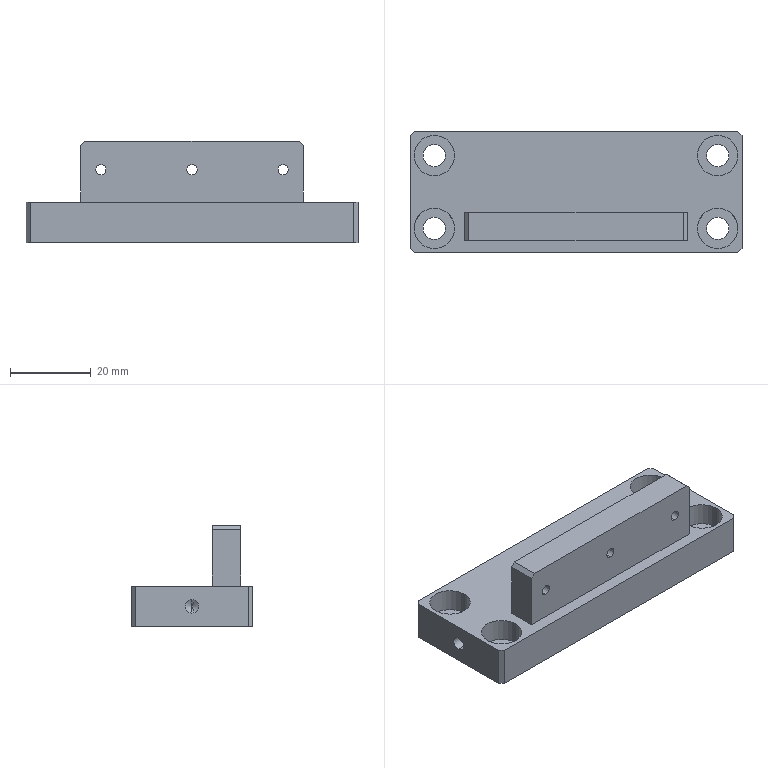Part | STEP file | 1 solid | 51 faces | box 82 x 30 x 25 mm | volume 27843 mm3 | cylinder 26 | plane 21 | cone 4 | commonest cylinder face diameters 5.5 x8 10 x8 2.5 x6 3.3 x4